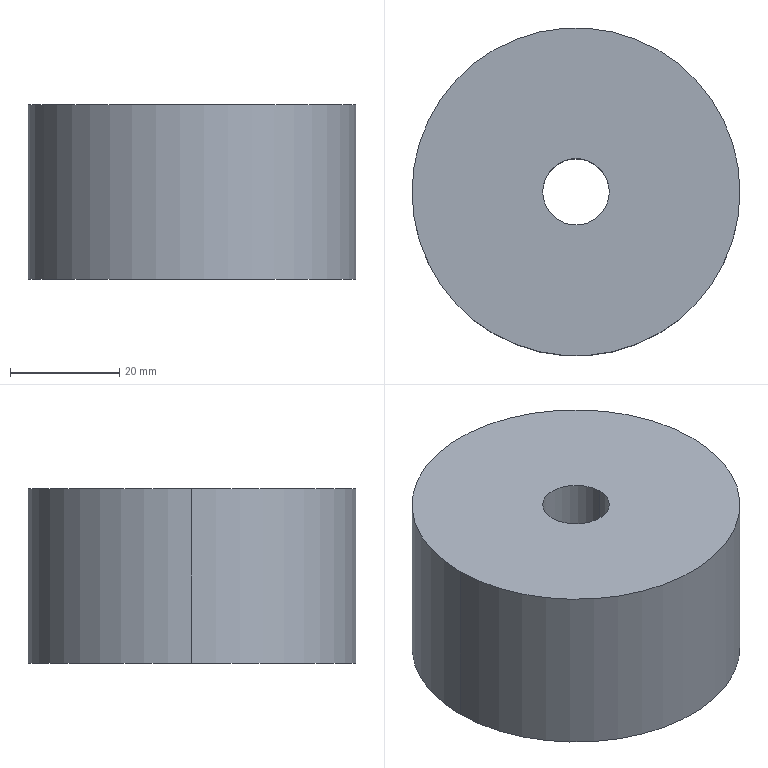Part | SolidWorks | features Extrusion 1 | 1 solid | 6 faces | box 60 x 60 x 32 mm | volume 86737 mm3 | cylinder 4 | plane 2 | commonest cylinder face diameters 12.2 x2 60 x2
STEP:
#1=CARTESIAN_POINT('',(-6.1,0.,-16.));
#2=VERTEX_POINT('',#1);
#3=CARTESIAN_POINT('',(6.1,0.,-16.));
#4=VERTEX_POINT('',#3);
#5=CARTESIAN_POINT('',(0.,0.,-16.));
#6=DIRECTION('',(0.,0.,1.));
#7=DIRECTION('',(1.,0.,0.));
#8=AXIS2_PLACEMENT_3D('',#5,#6,#7);
#9=CIRCLE('',#8,6.1);
#10=EDGE_CURVE('',#2,#4,#9,.T.);
#11=ORIENTED_EDGE('',*,*,#10,.F.);
#12=CARTESIAN_POINT('',(-6.1,0.,16.));
#13=VERTEX_POINT('',#12);
#14=CARTESIAN_POINT('',(-6.1,0.,-16.));
#15=DIRECTION('',(0.,0.,1.));
#16=VECTOR('',#15,1000.);
#17=LINE('',#14,#16);
#18=EDGE_CURVE('',#2,#13,#17,.T.);
#19=ORIENTED_EDGE('',*,*,#18,.T.);
#20=CARTESIAN_POINT('',(6.1,0.,16.));
#21=VERTEX_POINT('',#20);
#22=CARTESIAN_POINT('',(0.,0.,16.));
#23=DIRECTION('',(0.,0.,1.));
#24=DIRECTION('',(1.,0.,0.));
#25=AXIS2_PLACEMENT_3D('',#22,#23,#24);
#26=CIRCLE('',#25,6.1);
#27=EDGE_CURVE('',#13,#21,#26,.T.);
#28=ORIENTED_EDGE('',*,*,#27,.T.);
#29=CARTESIAN_POINT('',(6.1,0.,-16.));
#30=DIRECTION('',(0.,0.,1.));
#31=VECTOR('',#30,1000.);
#32=LINE('',#29,#31);
#33=EDGE_CURVE('',#4,#21,#32,.T.);
#34=ORIENTED_EDGE('',*,*,#33,.F.);
#35=EDGE_LOOP('',(#11,#19,#28,#34));
#36=FACE_OUTER_BOUND('',#35,.T.);
#37=CARTESIAN_POINT('',(0.,0.,-16.));
#38=DIRECTION('',(0.,0.,1.));
#39=DIRECTION('',(1.,0.,0.));
#40=AXIS2_PLACEMENT_3D('',#37,#38,#39);
#41=CYLINDRICAL_SURFACE('',#40,6.1);
#42=ADVANCED_FACE('',(#36),#41,.F.);
#43=CARTESIAN_POINT('',(30.,0.,-16.));
#44=VERTEX_POINT('',#43);
#45=CARTESIAN_POINT('',(-30.,0.,-16.));
#46=VERTEX_POINT('',#45);
#47=CARTESIAN_POINT('',(0.,0.,-16.));
#48=DIRECTION('',(0.,0.,1.));
#49=DIRECTION('',(1.,0.,0.));
#50=AXIS2_PLACEMENT_3D('',#47,#48,#49);
#51=CIRCLE('',#50,30.);
#52=EDGE_CURVE('',#44,#46,#51,.T.);
#53=ORIENTED_EDGE('',*,*,#52,.T.);
#54=CARTESIAN_POINT('',(-30.,0.,16.));
#55=VERTEX_POINT('',#54);
#56=CARTESIAN_POINT('',(-30.,0.,-16.));
#57=DIRECTION('',(0.,0.,1.));
#58=VECTOR('',#57,1000.);
#59=LINE('',#56,#58);
#60=EDGE_CURVE('',#46,#55,#59,.T.);
#61=ORIENTED_EDGE('',*,*,#60,.T.);
#62=CARTESIAN_POINT('',(30.,0.,16.));
#63=VERTEX_POINT('',#62);
#64=CARTESIAN_POINT('',(0.,0.,16.));
#65=DIRECTION('',(0.,0.,1.));
#66=DIRECTION('',(1.,0.,0.));
#67=AXIS2_PLACEMENT_3D('',#64,#65,#66);
#68=CIRCLE('',#67,30.);
#69=EDGE_CURVE('',#63,#55,#68,.T.);
#70=ORIENTED_EDGE('',*,*,#69,.F.);
#71=CARTESIAN_POINT('',(30.,0.,-16.));
#72=DIRECTION('',(0.,0.,1.));
#73=VECTOR('',#72,1000.);
#74=LINE('',#71,#73);
#75=EDGE_CURVE('',#44,#63,#74,.T.);
#76=ORIENTED_EDGE('',*,*,#75,.F.);
#77=EDGE_LOOP('',(#53,#61,#70,#76));
#78=FACE_OUTER_BOUND('',#77,.T.);
#79=CARTESIAN_POINT('',(0.,0.,-16.));
#80=DIRECTION('',(0.,0.,1.));
#81=DIRECTION('',(1.,0.,0.));
#82=AXIS2_PLACEMENT_3D('',#79,#80,#81);
#83=CYLINDRICAL_SURFACE('',#82,30.);
#84=ADVANCED_FACE('',(#78),#83,.T.);
#85=ORIENTED_EDGE('',*,*,#60,.F.);
#86=CARTESIAN_POINT('',(0.,0.,-16.));
#87=DIRECTION('',(0.,0.,1.));
#88=DIRECTION('',(1.,0.,0.));
#89=AXIS2_PLACEMENT_3D('',#86,#87,#88);
#90=CIRCLE('',#89,30.);
#91=EDGE_CURVE('',#46,#44,#90,.T.);
#92=ORIENTED_EDGE('',*,*,#91,.T.);
#93=ORIENTED_EDGE('',*,*,#75,.T.);
#94=CARTESIAN_POINT('',(0.,0.,16.));
#95=DIRECTION('',(0.,0.,1.));
#96=DIRECTION('',(1.,0.,0.));
#97=AXIS2_PLACEMENT_3D('',#94,#95,#96);
#98=CIRCLE('',#97,30.);
#99=EDGE_CURVE('',#55,#63,#98,.T.);
#100=ORIENTED_EDGE('',*,*,#99,.F.);
#101=EDGE_LOOP('',(#85,#92,#93,#100));
#102=FACE_OUTER_BOUND('',#101,.T.);
#103=CARTESIAN_POINT('',(0.,0.,-16.));
#104=DIRECTION('',(0.,0.,1.));
#105=DIRECTION('',(1.,0.,0.));
#106=AXIS2_PLACEMENT_3D('',#103,#104,#105);
#107=CYLINDRICAL_SURFACE('',#106,30.);
#108=ADVANCED_FACE('',(#102),#107,.T.);
#109=CARTESIAN_POINT('',(0.,0.,-16.));
#110=DIRECTION('',(0.,0.,1.));
#111=DIRECTION('',(1.,0.,0.));
#112=AXIS2_PLACEMENT_3D('',#109,#110,#111);
#113=CIRCLE('',#112,6.1);
#114=EDGE_CURVE('',#4,#2,#113,.T.);
#115=ORIENTED_EDGE('',*,*,#114,.T.);
#116=ORIENTED_EDGE('',*,*,#10,.T.);
#117=EDGE_LOOP('',(#115,#116));
#118=FACE_BOUND('',#117,.T.);
#119=ORIENTED_EDGE('',*,*,#52,.F.);
#120=ORIENTED_EDGE('',*,*,#91,.F.);
#121=EDGE_LOOP('',(#119,#120));
#122=FACE_OUTER_BOUND('',#121,.T.);
#123=CARTESIAN_POINT('',(0.,0.,-16.));
#124=DIRECTION('',(0.,0.,1.));
#125=DIRECTION('',(1.,0.,0.));
#126=AXIS2_PLACEMENT_3D('',#123,#124,#125);
#127=PLANE('',#126);
#128=ADVANCED_FACE('',(#118,#122),#127,.F.);
#129=CARTESIAN_POINT('',(0.,0.,16.));
#130=DIRECTION('',(0.,0.,1.));
#131=DIRECTION('',(1.,0.,0.));
#132=AXIS2_PLACEMENT_3D('',#129,#130,#131);
#133=CIRCLE('',#132,6.1);
#134=EDGE_CURVE('',#21,#13,#133,.T.);
#135=ORIENTED_EDGE('',*,*,#134,.F.);
#136=ORIENTED_EDGE('',*,*,#27,.F.);
#137=EDGE_LOOP('',(#135,#136));
#138=FACE_BOUND('',#137,.T.);
#139=ORIENTED_EDGE('',*,*,#69,.T.);
#140=ORIENTED_EDGE('',*,*,#99,.T.);
#141=EDGE_LOOP('',(#139,#140));
#142=FACE_OUTER_BOUND('',#141,.T.);
#143=CARTESIAN_POINT('',(0.,0.,16.));
#144=DIRECTION('',(0.,0.,1.));
#145=DIRECTION('',(1.,0.,0.));
#146=AXIS2_PLACEMENT_3D('',#143,#144,#145);
#147=PLANE('',#146);
#148=ADVANCED_FACE('',(#138,#142),#147,.T.);
#149=ORIENTED_EDGE('',*,*,#18,.F.);
#150=ORIENTED_EDGE('',*,*,#114,.F.);
#151=ORIENTED_EDGE('',*,*,#33,.T.);
#152=ORIENTED_EDGE('',*,*,#134,.T.);
#153=EDGE_LOOP('',(#149,#150,#151,#152));
#154=FACE_OUTER_BOUND('',#153,.T.);
#155=CARTESIAN_POINT('',(0.,0.,-16.));
#156=DIRECTION('',(0.,0.,1.));
#157=DIRECTION('',(1.,0.,0.));
#158=AXIS2_PLACEMENT_3D('',#155,#156,#157);
#159=CYLINDRICAL_SURFACE('',#158,6.1);
#160=ADVANCED_FACE('',(#154),#159,.F.);
#161=CLOSED_SHELL('',(#42,#84,#108,#128,#148,#160));
#162=MANIFOLD_SOLID_BREP('',#161);
#163=CARTESIAN_POINT('',(0.,0.,0.));
#164=DIRECTION('',(0.,0.,1.));
#165=DIRECTION('',(1.,0.,0.));
#166=AXIS2_PLACEMENT_3D('',#163,#164,#165);
#167=(LENGTH_UNIT()NAMED_UNIT(*)SI_UNIT(.MILLI.,.METRE.));
#168=UNCERTAINTY_MEASURE_WITH_UNIT(LENGTH_MEASURE(0.00001),#167,'','');
#169=(NAMED_UNIT(*)PLANE_ANGLE_UNIT()SI_UNIT($,.RADIAN.));
#170=(NAMED_UNIT(*)SI_UNIT($,.STERADIAN.)SOLID_ANGLE_UNIT());
#171=(GEOMETRIC_REPRESENTATION_CONTEXT(3)GLOBAL_UNCERTAINTY_ASSIGNED_CONTEXT((#168))GLOBAL_UNIT_ASSIGNED_CONTEXT((#167,#169,#170))REPRESENTATION_CONTEXT('',''));
#172=ADVANCED_BREP_SHAPE_REPRESENTATION('',(#162,#166),#171);